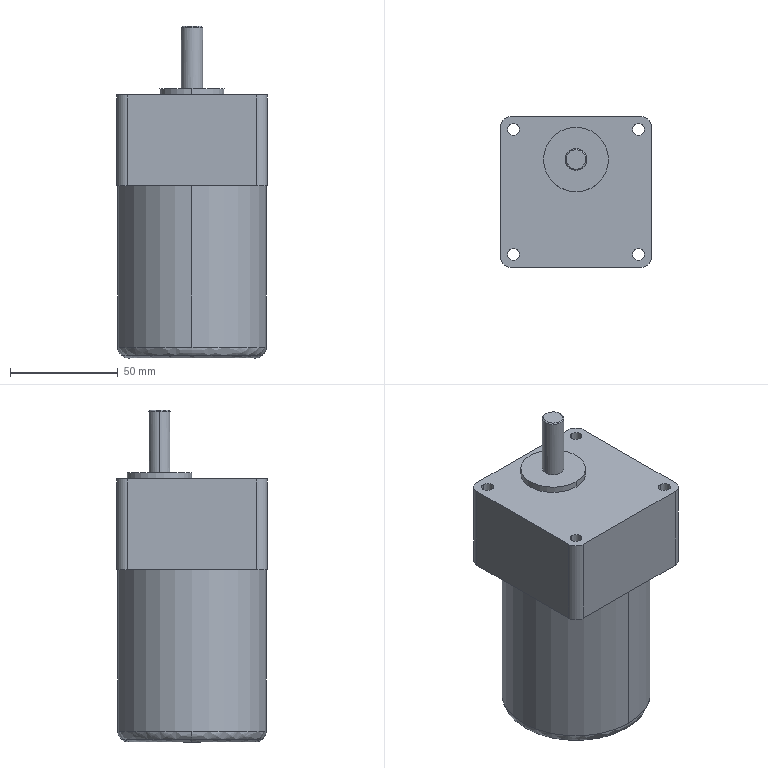Part | SolidWorks | features BaseBody 1 | 1 solid | 33 faces | box 70 x 70 x 154 mm | volume 503318 mm3 | cylinder 18 | plane 9 | spline 4 | cone 2 | commonest cylinder face diameters 5.5 x8 10 x6 30 x2 69 x2
STEP:
#1=CARTESIAN_POINT('',(180.25,352.,-74.5));
#2=VERTEX_POINT('',#1);
#3=CARTESIAN_POINT('',(239.25,352.,-74.5));
#4=VERTEX_POINT('',#3);
#5=CARTESIAN_POINT('',(180.25,352.,-74.5));
#6=CARTESIAN_POINT('',(180.25,353.933,-74.5));
#7=CARTESIAN_POINT('',(180.44,355.861,-74.5));
#8=CARTESIAN_POINT('',(181.194,359.65,-74.5));
#9=CARTESIAN_POINT('',(181.756,361.505,-74.5));
#10=CARTESIAN_POINT('',(183.235,365.074,-74.5));
#11=CARTESIAN_POINT('',(184.149,366.783,-74.5));
#12=CARTESIAN_POINT('',(186.295,369.995,-74.5));
#13=CARTESIAN_POINT('',(187.525,371.494,-74.5));
#14=CARTESIAN_POINT('',(190.256,374.226,-74.5));
#15=CARTESIAN_POINT('',(191.755,375.455,-74.5));
#16=CARTESIAN_POINT('',(194.967,377.602,-74.5));
#17=CARTESIAN_POINT('',(196.676,378.515,-74.5));
#18=CARTESIAN_POINT('',(200.245,379.994,-74.5));
#19=CARTESIAN_POINT('',(202.1,380.556,-74.5));
#20=CARTESIAN_POINT('',(205.889,381.31,-74.5));
#21=CARTESIAN_POINT('',(207.818,381.5,-74.5));
#22=CARTESIAN_POINT('',(211.682,381.5,-74.5));
#23=CARTESIAN_POINT('',(213.611,381.31,-74.5));
#24=CARTESIAN_POINT('',(217.4,380.556,-74.5));
#25=CARTESIAN_POINT('',(219.255,379.994,-74.5));
#26=CARTESIAN_POINT('',(222.824,378.515,-74.5));
#27=CARTESIAN_POINT('',(224.533,377.601,-74.5));
#28=CARTESIAN_POINT('',(227.745,375.455,-74.5));
#29=CARTESIAN_POINT('',(229.244,374.225,-74.5));
#30=CARTESIAN_POINT('',(231.976,371.494,-74.5));
#31=CARTESIAN_POINT('',(233.205,369.995,-74.5));
#32=CARTESIAN_POINT('',(235.352,366.783,-74.5));
#33=CARTESIAN_POINT('',(236.265,365.074,-74.5));
#34=CARTESIAN_POINT('',(237.744,361.505,-74.5));
#35=CARTESIAN_POINT('',(238.306,359.65,-74.5));
#36=CARTESIAN_POINT('',(239.06,355.861,-74.5));
#37=CARTESIAN_POINT('',(239.25,353.933,-74.5));
#38=CARTESIAN_POINT('',(239.25,352.,-74.5));
#39=B_SPLINE_CURVE_WITH_KNOTS('',3,(#5,#6,#7,#8,#9,#10,#11,#12,#13,#14,#15,#16,#17,#18,#19,#20,#21,#22,#23,#24,#25,#26,#27,#28,#29,#30,#31,#32,#33,#34,#35,#36,#37,#38),.UNSPECIFIED.,.F.,.F.,(4,2,2,2,2,2,2,2,2,2,2,2,2,2,2,2,4),(0.,0.0625,0.125,0.1875,0.25,0.3125,0.375,0.4375,0.5,0.5625,0.625,0.6875,0.75,0.8125,0.875,0.9375,1.),.UNSPECIFIED.);
#40=EDGE_CURVE('',#2,#4,#39,.T.);
#41=ORIENTED_EDGE('',*,*,#40,.F.);
#42=CARTESIAN_POINT('',(176.873,352.,-73.187));
#43=VERTEX_POINT('',#42);
#44=CARTESIAN_POINT('',(180.25,352.,-69.5));
#45=DIRECTION('',(0.,1.,0.));
#46=DIRECTION('',(-0.6754,0.,-0.7375));
#47=AXIS2_PLACEMENT_3D('',#44,#45,#46);
#48=CIRCLE('',#47,5.);
#49=EDGE_CURVE('',#2,#43,#48,.T.);
#50=ORIENTED_EDGE('',*,*,#49,.T.);
#51=CARTESIAN_POINT('',(242.627,352.,-73.187));
#52=VERTEX_POINT('',#51);
#53=CARTESIAN_POINT('',(209.75,352.,-73.187));
#54=DIRECTION('',(0.,0.,1.));
#55=DIRECTION('',(1.,0.,0.));
#56=AXIS2_PLACEMENT_3D('',#53,#54,#55);
#57=CIRCLE('',#56,32.877);
#58=EDGE_CURVE('',#52,#43,#57,.T.);
#59=ORIENTED_EDGE('',*,*,#58,.F.);
#60=CARTESIAN_POINT('',(239.25,352.,-69.5));
#61=DIRECTION('',(0.,-1.,0.));
#62=DIRECTION('',(0.6754,0.,-0.7375));
#63=AXIS2_PLACEMENT_3D('',#60,#61,#62);
#64=CIRCLE('',#63,5.);
#65=EDGE_CURVE('',#4,#52,#64,.T.);
#66=ORIENTED_EDGE('',*,*,#65,.F.);
#67=EDGE_LOOP('',(#41,#50,#59,#66));
#68=FACE_OUTER_BOUND('',#67,.T.);
#69=CARTESIAN_POINT('',(239.25,352.,-74.5));
#70=CARTESIAN_POINT('',(239.25,411.,-74.5));
#71=CARTESIAN_POINT('',(180.25,411.,-74.5));
#72=CARTESIAN_POINT('',(180.25,352.,-74.5));
#73=CARTESIAN_POINT('',(240.515,352.,-74.5));
#74=CARTESIAN_POINT('',(240.515,413.53,-74.5));
#75=CARTESIAN_POINT('',(178.985,413.53,-74.5));
#76=CARTESIAN_POINT('',(178.985,352.,-74.5));
#77=CARTESIAN_POINT('',(241.694,352.,-74.042));
#78=CARTESIAN_POINT('',(241.694,415.888,-74.042));
#79=CARTESIAN_POINT('',(177.806,415.888,-74.042));
#80=CARTESIAN_POINT('',(177.806,352.,-74.042));
#81=CARTESIAN_POINT('',(242.627,352.,-73.187));
#82=CARTESIAN_POINT('',(242.627,417.754,-73.187));
#83=CARTESIAN_POINT('',(176.873,417.754,-73.187));
#84=CARTESIAN_POINT('',(176.873,352.,-73.187));
#85=(BOUNDED_SURFACE()B_SPLINE_SURFACE(3,3,((#69,#70,#71,#72),(#73,#74,#75,#76),(#77,#78,#79,#80),(#81,#82,#83,#84)),.UNSPECIFIED.,.F.,.F.,.F.)B_SPLINE_SURFACE_WITH_KNOTS((4,4),(4,4),(0.,1.),(0.,1.),.UNSPECIFIED.)GEOMETRIC_REPRESENTATION_ITEM()RATIONAL_B_SPLINE_SURFACE(((1.,0.3333,0.3333,1.),(0.9547,0.3182,0.3182,0.9547),(0.9547,0.3182,0.3182,0.9547),(1.,0.3333,0.3333,1.)))REPRESENTATION_ITEM('')SURFACE());
#86=ADVANCED_FACE('',(#68),#85,.F.);
#87=ORIENTED_EDGE('',*,*,#58,.T.);
#88=CARTESIAN_POINT('',(175.25,352.,-69.5));
#89=VERTEX_POINT('',#88);
#90=CARTESIAN_POINT('',(180.25,352.,-69.5));
#91=DIRECTION('',(0.,1.,0.));
#92=DIRECTION('',(-0.6754,0.,-0.7375));
#93=AXIS2_PLACEMENT_3D('',#90,#91,#92);
#94=CIRCLE('',#93,5.);
#95=EDGE_CURVE('',#43,#89,#94,.T.);
#96=ORIENTED_EDGE('',*,*,#95,.T.);
#97=CARTESIAN_POINT('',(209.75,386.5,-69.5));
#98=VERTEX_POINT('',#97);
#99=CARTESIAN_POINT('',(209.75,352.,-69.5));
#100=DIRECTION('',(0.,0.,-1.));
#101=DIRECTION('',(1.,0.,0.));
#102=AXIS2_PLACEMENT_3D('',#99,#100,#101);
#103=CIRCLE('',#102,34.5);
#104=EDGE_CURVE('',#89,#98,#103,.T.);
#105=ORIENTED_EDGE('',*,*,#104,.T.);
#106=CARTESIAN_POINT('',(244.25,352.,-69.5));
#107=VERTEX_POINT('',#106);
#108=CARTESIAN_POINT('',(209.75,352.,-69.5));
#109=DIRECTION('',(0.,0.,-1.));
#110=DIRECTION('',(1.,0.,0.));
#111=AXIS2_PLACEMENT_3D('',#108,#109,#110);
#112=CIRCLE('',#111,34.5);
#113=EDGE_CURVE('',#98,#107,#112,.T.);
#114=ORIENTED_EDGE('',*,*,#113,.T.);
#115=CARTESIAN_POINT('',(239.25,352.,-69.5));
#116=DIRECTION('',(0.,-1.,0.));
#117=DIRECTION('',(0.6754,0.,-0.7375));
#118=AXIS2_PLACEMENT_3D('',#115,#116,#117);
#119=CIRCLE('',#118,5.);
#120=EDGE_CURVE('',#52,#107,#119,.T.);
#121=ORIENTED_EDGE('',*,*,#120,.F.);
#122=EDGE_LOOP('',(#87,#96,#105,#114,#121));
#123=FACE_OUTER_BOUND('',#122,.T.);
#124=CARTESIAN_POINT('',(242.627,352.,-73.187));
#125=CARTESIAN_POINT('',(242.627,417.754,-73.187));
#126=CARTESIAN_POINT('',(176.873,417.754,-73.187));
#127=CARTESIAN_POINT('',(176.873,352.,-73.187));
#128=CARTESIAN_POINT('',(243.677,352.,-72.226));
#129=CARTESIAN_POINT('',(243.677,419.853,-72.226));
#130=CARTESIAN_POINT('',(175.823,419.853,-72.226));
#131=CARTESIAN_POINT('',(175.823,352.,-72.226));
#132=CARTESIAN_POINT('',(244.25,352.,-70.923));
#133=CARTESIAN_POINT('',(244.25,421.,-70.923));
#134=CARTESIAN_POINT('',(175.25,421.,-70.923));
#135=CARTESIAN_POINT('',(175.25,352.,-70.923));
#136=CARTESIAN_POINT('',(244.25,352.,-69.5));
#137=CARTESIAN_POINT('',(244.25,421.,-69.5));
#138=CARTESIAN_POINT('',(175.25,421.,-69.5));
#139=CARTESIAN_POINT('',(175.25,352.,-69.5));
#140=(BOUNDED_SURFACE()B_SPLINE_SURFACE(3,3,((#124,#125,#126,#127),(#128,#129,#130,#131),(#132,#133,#134,#135),(#136,#137,#138,#139)),.UNSPECIFIED.,.F.,.F.,.F.)B_SPLINE_SURFACE_WITH_KNOTS((4,4),(4,4),(0.,1.),(0.,1.),.UNSPECIFIED.)GEOMETRIC_REPRESENTATION_ITEM()RATIONAL_B_SPLINE_SURFACE(((1.,0.3333,0.3333,1.),(0.9435,0.3145,0.3145,0.9435),(0.9435,0.3145,0.3145,0.9435),(1.,0.3333,0.3333,1.)))REPRESENTATION_ITEM('')SURFACE());
#141=ADVANCED_FACE('',(#123),#140,.F.);
#142=CARTESIAN_POINT('',(209.75,362.5,79.5));
#143=VERTEX_POINT('',#142);
#144=CARTESIAN_POINT('',(209.75,371.5,79.5));
#145=VERTEX_POINT('',#144);
#146=CARTESIAN_POINT('',(209.75,367.,79.5));
#147=DIRECTION('',(0.,0.,1.));
#148=DIRECTION('',(0.,1.,0.));
#149=AXIS2_PLACEMENT_3D('',#146,#147,#148);
#150=CIRCLE('',#149,4.5);
#151=EDGE_CURVE('',#143,#145,#150,.T.);
#152=ORIENTED_EDGE('',*,*,#151,.F.);
#153=CARTESIAN_POINT('',(209.75,362.,79.));
#154=VERTEX_POINT('',#153);
#155=CARTESIAN_POINT('',(209.75,362.5,79.5));
#156=DIRECTION('',(0.,-0.7071,-0.7071));
#157=VECTOR('',#156,1000.);
#158=LINE('',#155,#157);
#159=EDGE_CURVE('',#143,#154,#158,.T.);
#160=ORIENTED_EDGE('',*,*,#159,.T.);
#161=CARTESIAN_POINT('',(214.75,367.,79.));
#162=VERTEX_POINT('',#161);
#163=CARTESIAN_POINT('',(209.75,367.,79.));
#164=DIRECTION('',(0.,0.,-1.));
#165=DIRECTION('',(-1.,0.,0.));
#166=AXIS2_PLACEMENT_3D('',#163,#164,#165);
#167=CIRCLE('',#166,5.);
#168=EDGE_CURVE('',#162,#154,#167,.T.);
#169=ORIENTED_EDGE('',*,*,#168,.F.);
#170=CARTESIAN_POINT('',(209.75,372.,79.));
#171=VERTEX_POINT('',#170);
#172=CARTESIAN_POINT('',(209.75,367.,79.));
#173=DIRECTION('',(0.,0.,-1.));
#174=DIRECTION('',(-1.,0.,0.));
#175=AXIS2_PLACEMENT_3D('',#172,#173,#174);
#176=CIRCLE('',#175,5.);
#177=EDGE_CURVE('',#171,#162,#176,.T.);
#178=ORIENTED_EDGE('',*,*,#177,.F.);
#179=CARTESIAN_POINT('',(209.75,371.5,79.5));
#180=DIRECTION('',(0.,0.7071,-0.7071));
#181=VECTOR('',#180,1000.);
#182=LINE('',#179,#181);
#183=EDGE_CURVE('',#145,#171,#182,.T.);
#184=ORIENTED_EDGE('',*,*,#183,.F.);
#185=EDGE_LOOP('',(#152,#160,#169,#178,#184));
#186=FACE_OUTER_BOUND('',#185,.T.);
#187=CARTESIAN_POINT('',(209.75,367.,79.5));
#188=DIRECTION('',(0.,0.,-1.));
#189=DIRECTION('',(0.,1.,0.));
#190=AXIS2_PLACEMENT_3D('',#187,#188,#189);
#191=CONICAL_SURFACE('',#190,4.5,0.7854);
#192=ADVANCED_FACE('',(#186),#191,.T.);
#193=CARTESIAN_POINT('',(204.75,367.,50.5));
#194=VERTEX_POINT('',#193);
#195=CARTESIAN_POINT('',(214.75,367.,50.5));
#196=VERTEX_POINT('',#195);
#197=CARTESIAN_POINT('',(209.75,367.,50.5));
#198=DIRECTION('',(0.,0.,-1.));
#199=DIRECTION('',(1.,0.,0.));
#200=AXIS2_PLACEMENT_3D('',#197,#198,#199);
#201=CIRCLE('',#200,5.);
#202=EDGE_CURVE('',#194,#196,#201,.T.);
#203=ORIENTED_EDGE('',*,*,#202,.F.);
#204=CARTESIAN_POINT('',(204.75,367.,79.));
#205=VERTEX_POINT('',#204);
#206=CARTESIAN_POINT('',(204.75,367.,50.5));
#207=DIRECTION('',(0.,0.,1.));
#208=VECTOR('',#207,1000.);
#209=LINE('',#206,#208);
#210=EDGE_CURVE('',#194,#205,#209,.T.);
#211=ORIENTED_EDGE('',*,*,#210,.T.);
#212=CARTESIAN_POINT('',(209.75,367.,79.));
#213=DIRECTION('',(0.,0.,-1.));
#214=DIRECTION('',(-1.,0.,0.));
#215=AXIS2_PLACEMENT_3D('',#212,#213,#214);
#216=CIRCLE('',#215,5.);
#217=EDGE_CURVE('',#205,#171,#216,.T.);
#218=ORIENTED_EDGE('',*,*,#217,.T.);
#219=ORIENTED_EDGE('',*,*,#177,.T.);
#220=CARTESIAN_POINT('',(214.75,367.,50.5));
#221=DIRECTION('',(0.,0.,1.));
#222=VECTOR('',#221,1000.);
#223=LINE('',#220,#222);
#224=EDGE_CURVE('',#196,#162,#223,.T.);
#225=ORIENTED_EDGE('',*,*,#224,.F.);
#226=EDGE_LOOP('',(#203,#211,#218,#219,#225));
#227=FACE_OUTER_BOUND('',#226,.T.);
#228=CARTESIAN_POINT('',(209.75,367.,50.5));
#229=DIRECTION('',(0.,0.,1.));
#230=DIRECTION('',(1.,0.,0.));
#231=AXIS2_PLACEMENT_3D('',#228,#229,#230);
#232=CYLINDRICAL_SURFACE('',#231,5.);
#233=ADVANCED_FACE('',(#227),#232,.T.);
#234=CARTESIAN_POINT('',(209.75,382.,47.5));
#235=VERTEX_POINT('',#234);
#236=CARTESIAN_POINT('',(209.75,352.,47.5));
#237=VERTEX_POINT('',#236);
#238=CARTESIAN_POINT('',(209.75,367.,47.5));
#239=DIRECTION('',(0.,0.,-1.));
#240=DIRECTION('',(0.,-1.,0.));
#241=AXIS2_PLACEMENT_3D('',#238,#239,#240);
#242=CIRCLE('',#241,15.);
#243=EDGE_CURVE('',#235,#237,#242,.T.);
#244=ORIENTED_EDGE('',*,*,#243,.F.);
#245=CARTESIAN_POINT('',(209.75,382.,50.5));
#246=VERTEX_POINT('',#245);
#247=CARTESIAN_POINT('',(209.75,382.,47.5));
#248=DIRECTION('',(0.,0.,1.));
#249=VECTOR('',#248,1000.);
#250=LINE('',#247,#249);
#251=EDGE_CURVE('',#235,#246,#250,.T.);
#252=ORIENTED_EDGE('',*,*,#251,.T.);
#253=CARTESIAN_POINT('',(209.75,352.,50.5));
#254=VERTEX_POINT('',#253);
#255=CARTESIAN_POINT('',(209.75,367.,50.5));
#256=DIRECTION('',(0.,0.,-1.));
#257=DIRECTION('',(0.,-1.,0.));
#258=AXIS2_PLACEMENT_3D('',#255,#256,#257);
#259=CIRCLE('',#258,15.);
#260=EDGE_CURVE('',#246,#254,#259,.T.);
#261=ORIENTED_EDGE('',*,*,#260,.T.);
#262=CARTESIAN_POINT('',(209.75,352.,47.5));
#263=DIRECTION('',(0.,0.,1.));
#264=VECTOR('',#263,1000.);
#265=LINE('',#262,#264);
#266=EDGE_CURVE('',#237,#254,#265,.T.);
#267=ORIENTED_EDGE('',*,*,#266,.F.);
#268=EDGE_LOOP('',(#244,#252,#261,#267));
#269=FACE_OUTER_BOUND('',#268,.T.);
#270=CARTESIAN_POINT('',(209.75,367.,47.5));
#271=DIRECTION('',(0.,0.,1.));
#272=DIRECTION('',(0.,-1.,0.));
#273=AXIS2_PLACEMENT_3D('',#270,#271,#272);
#274=CYLINDRICAL_SURFACE('',#273,15.);
#275=ADVANCED_FACE('',(#269),#274,.T.);
#276=CARTESIAN_POINT('',(238.741,378.241,47.5));
#277=VERTEX_POINT('',#276);
#278=CARTESIAN_POINT('',(238.741,383.741,47.5));
#279=VERTEX_POINT('',#278);
#280=CARTESIAN_POINT('',(238.741,380.991,47.5));
#281=DIRECTION('',(0.,0.,-1.));
#282=DIRECTION('',(0.,1.,0.));
#283=AXIS2_PLACEMENT_3D('',#280,#281,#282);
#284=CIRCLE('',#283,2.75);
#285=EDGE_CURVE('',#277,#279,#284,.T.);
#286=ORIENTED_EDGE('',*,*,#285,.F.);
#287=CARTESIAN_POINT('',(238.741,378.241,5.5));
#288=VERTEX_POINT('',#287);
#289=CARTESIAN_POINT('',(238.741,378.241,47.5));
#290=DIRECTION('',(0.,0.,-1.));
#291=VECTOR('',#290,1000.);
#292=LINE('',#289,#291);
#293=EDGE_CURVE('',#277,#288,#292,.T.);
#294=ORIENTED_EDGE('',*,*,#293,.T.);
#295=CARTESIAN_POINT('',(238.741,383.741,5.5));
#296=VERTEX_POINT('',#295);
#297=CARTESIAN_POINT('',(238.741,380.991,5.5));
#298=DIRECTION('',(0.,0.,-1.));
#299=DIRECTION('',(0.,1.,0.));
#300=AXIS2_PLACEMENT_3D('',#297,#298,#299);
#301=CIRCLE('',#300,2.75);
#302=EDGE_CURVE('',#288,#296,#301,.T.);
#303=ORIENTED_EDGE('',*,*,#302,.T.);
#304=CARTESIAN_POINT('',(238.741,383.741,47.5));
#305=DIRECTION('',(0.,0.,-1.));
#306=VECTOR('',#305,1000.);
#307=LINE('',#304,#306);
#308=EDGE_CURVE('',#279,#296,#307,.T.);
#309=ORIENTED_EDGE('',*,*,#308,.F.);
#310=EDGE_LOOP('',(#286,#294,#303,#309));
#311=FACE_OUTER_BOUND('',#310,.T.);
#312=CARTESIAN_POINT('',(238.741,380.991,47.5));
#313=DIRECTION('',(0.,0.,-1.));
#314=DIRECTION('',(0.,1.,0.));
#315=AXIS2_PLACEMENT_3D('',#312,#313,#314);
#316=CYLINDRICAL_SURFACE('',#315,2.75);
#317=ADVANCED_FACE('',(#311),#316,.F.);
#318=CARTESIAN_POINT('',(238.741,320.259,47.5));
#319=VERTEX_POINT('',#318);
#320=CARTESIAN_POINT('',(238.741,325.759,47.5));
#321=VERTEX_POINT('',#320);
#322=CARTESIAN_POINT('',(238.741,323.009,47.5));
#323=DIRECTION('',(0.,0.,-1.));
#324=DIRECTION('',(0.,1.,0.));
#325=AXIS2_PLACEMENT_3D('',#322,#323,#324);
#326=CIRCLE('',#325,2.75);
#327=EDGE_CURVE('',#319,#321,#326,.T.);
#328=ORIENTED_EDGE('',*,*,#327,.F.);
#329=CARTESIAN_POINT('',(238.741,320.259,5.5));
#330=VERTEX_POINT('',#329);
#331=CARTESIAN_POINT('',(238.741,320.259,47.5));
#332=DIRECTION('',(0.,0.,-1.));
#333=VECTOR('',#332,1000.);
#334=LINE('',#331,#333);
#335=EDGE_CURVE('',#319,#330,#334,.T.);
#336=ORIENTED_EDGE('',*,*,#335,.T.);
#337=CARTESIAN_POINT('',(238.741,325.759,5.5));
#338=VERTEX_POINT('',#337);
#339=CARTESIAN_POINT('',(238.741,323.009,5.5));
#340=DIRECTION('',(0.,0.,-1.));
#341=DIRECTION('',(0.,1.,0.));
#342=AXIS2_PLACEMENT_3D('',#339,#340,#341);
#343=CIRCLE('',#342,2.75);
#344=EDGE_CURVE('',#330,#338,#343,.T.);
#345=ORIENTED_EDGE('',*,*,#344,.T.);
#346=CARTESIAN_POINT('',(238.741,325.759,47.5));
#347=DIRECTION('',(0.,0.,-1.));
#348=VECTOR('',#347,1000.);
#349=LINE('',#346,#348);
#350=EDGE_CURVE('',#321,#338,#349,.T.);
#351=ORIENTED_EDGE('',*,*,#350,.F.);
#352=EDGE_LOOP('',(#328,#336,#345,#351));
#353=FACE_OUTER_BOUND('',#352,.T.);
#354=CARTESIAN_POINT('',(238.741,323.009,47.5));
#355=DIRECTION('',(0.,0.,-1.));
#356=DIRECTION('',(0.,1.,0.));
#357=AXIS2_PLACEMENT_3D('',#354,#355,#356);
#358=CYLINDRICAL_SURFACE('',#357,2.75);
#359=ADVANCED_FACE('',(#353),#358,.F.);
#360=CARTESIAN_POINT('',(180.759,320.259,47.5));
#361=VERTEX_POINT('',#360);
#362=CARTESIAN_POINT('',(180.759,325.759,47.5));
#363=VERTEX_POINT('',#362);
#364=CARTESIAN_POINT('',(180.759,323.009,47.5));
#365=DIRECTION('',(0.,0.,-1.));
#366=DIRECTION('',(0.,1.,0.));
#367=AXIS2_PLACEMENT_3D('',#364,#365,#366);
#368=CIRCLE('',#367,2.75);
#369=EDGE_CURVE('',#361,#363,#368,.T.);
#370=ORIENTED_EDGE('',*,*,#369,.F.);
#371=CARTESIAN_POINT('',(180.759,320.259,5.5));
#372=VERTEX_POINT('',#371);
#373=CARTESIAN_POINT('',(180.759,320.259,47.5));
#374=DIRECTION('',(0.,0.,-1.));
#375=VECTOR('',#374,1000.);
#376=LINE('',#373,#375);
#377=EDGE_CURVE('',#361,#372,#376,.T.);
#378=ORIENTED_EDGE('',*,*,#377,.T.);
#379=CARTESIAN_POINT('',(180.759,325.759,5.5));
#380=VERTEX_POINT('',#379);
#381=CARTESIAN_POINT('',(180.759,323.009,5.5));
#382=DIRECTION('',(0.,0.,-1.));
#383=DIRECTION('',(0.,1.,0.));
#384=AXIS2_PLACEMENT_3D('',#381,#382,#383);
#385=CIRCLE('',#384,2.75);
#386=EDGE_CURVE('',#372,#380,#385,.T.);
#387=ORIENTED_EDGE('',*,*,#386,.T.);
#388=CARTESIAN_POINT('',(180.759,325.759,47.5));
#389=DIRECTION('',(0.,0.,-1.));
#390=VECTOR('',#389,1000.);
#391=LINE('',#388,#390);
#392=EDGE_CURVE('',#363,#380,#391,.T.);
#393=ORIENTED_EDGE('',*,*,#392,.F.);
#394=EDGE_LOOP('',(#370,#378,#387,#393));
#395=FACE_OUTER_BOUND('',#394,.T.);
#396=CARTESIAN_POINT('',(180.759,323.009,47.5));
#397=DIRECTION('',(0.,0.,-1.));
#398=DIRECTION('',(0.,1.,0.));
#399=AXIS2_PLACEMENT_3D('',#396,#397,#398);
#400=CYLINDRICAL_SURFACE('',#399,2.75);
#401=ADVANCED_FACE('',(#395),#400,.F.);
#402=CARTESIAN_POINT('',(180.759,378.241,47.5));
#403=VERTEX_POINT('',#402);
#404=CARTESIAN_POINT('',(180.759,383.741,47.5));
#405=VERTEX_POINT('',#404);
#406=CARTESIAN_POINT('',(180.759,380.991,47.5));
#407=DIRECTION('',(0.,0.,-1.));
#408=DIRECTION('',(0.,1.,0.));
#409=AXIS2_PLACEMENT_3D('',#406,#407,#408);
#410=CIRCLE('',#409,2.75);
#411=EDGE_CURVE('',#403,#405,#410,.T.);
#412=ORIENTED_EDGE('',*,*,#411,.F.);
#413=CARTESIAN_POINT('',(180.759,378.241,5.5));
#414=VERTEX_POINT('',#413);
#415=CARTESIAN_POINT('',(180.759,378.241,47.5));
#416=DIRECTION('',(0.,0.,-1.));
#417=VECTOR('',#416,1000.);
#418=LINE('',#415,#417);
#419=EDGE_CURVE('',#403,#414,#418,.T.);
#420=ORIENTED_EDGE('',*,*,#419,.T.);
#421=CARTESIAN_POINT('',(180.759,383.741,5.5));
#422=VERTEX_POINT('',#421);
#423=CARTESIAN_POINT('',(180.759,380.991,5.5));
#424=DIRECTION('',(0.,0.,-1.));
#425=DIRECTION('',(0.,1.,0.));
#426=AXIS2_PLACEMENT_3D('',#423,#424,#425);
#427=CIRCLE('',#426,2.75);
#428=EDGE_CURVE('',#414,#422,#427,.T.);
#429=ORIENTED_EDGE('',*,*,#428,.T.);
#430=CARTESIAN_POINT('',(180.759,383.741,47.5));
#431=DIRECTION('',(0.,0.,-1.));
#432=VECTOR('',#431,1000.);
#433=LINE('',#430,#432);
#434=EDGE_CURVE('',#405,#422,#433,.T.);
#435=ORIENTED_EDGE('',*,*,#434,.F.);
#436=EDGE_LOOP('',(#412,#420,#429,#435));
#437=FACE_OUTER_BOUND('',#436,.T.);
#438=CARTESIAN_POINT('',(180.759,380.991,47.5));
#439=DIRECTION('',(0.,0.,-1.));
#440=DIRECTION('',(0.,1.,0.));
#441=AXIS2_PLACEMENT_3D('',#438,#439,#440);
#442=CYLINDRICAL_SURFACE('',#441,2.75);
#443=ADVANCED_FACE('',(#437),#442,.F.);
#444=CARTESIAN_POINT('',(209.75,386.5,5.5));
#445=VERTEX_POINT('',#444);
#446=CARTESIAN_POINT('',(209.75,317.5,5.5));
#447=VERTEX_POINT('',#446);
#448=CARTESIAN_POINT('',(209.75,352.,5.5));
#449=DIRECTION('',(0.,0.,-1.));
#450=DIRECTION('',(0.,1.,0.));
#451=AXIS2_PLACEMENT_3D('',#448,#449,#450);
#452=CIRCLE('',#451,34.5);
#453=EDGE_CURVE('',#445,#447,#452,.T.);
#454=ORIENTED_EDGE('',*,*,#453,.T.);
#455=CARTESIAN_POINT('',(209.75,317.5,-69.5));
#456=VERTEX_POINT('',#455);
#457=CARTESIAN_POINT('',(209.75,317.5,5.5));
#458=DIRECTION('',(0.,0.,-1.));
#459=VECTOR('',#458,1000.);
#460=LINE('',#457,#459);
#461=EDGE_CURVE('',#447,#456,#460,.T.);
#462=ORIENTED_EDGE('',*,*,#461,.T.);
#463=CARTESIAN_POINT('',(209.75,352.,-69.5));
#464=DIRECTION('',(0.,0.,-1.));
#465=DIRECTION('',(1.,0.,0.));
#466=AXIS2_PLACEMENT_3D('',#463,#464,#465);
#467=CIRCLE('',#466,34.5);
#468=EDGE_CURVE('',#107,#456,#467,.T.);
#469=ORIENTED_EDGE('',*,*,#468,.F.);
#470=ORIENTED_EDGE('',*,*,#113,.F.);
#471=CARTESIAN_POINT('',(209.75,386.5,5.5));
#472=DIRECTION('',(0.,0.,-1.));
#473=VECTOR('',#472,1000.);
#474=LINE('',#471,#473);
#475=EDGE_CURVE('',#445,#98,#474,.T.);
#476=ORIENTED_EDGE('',*,*,#475,.F.);
#477=EDGE_LOOP('',(#454,#462,#469,#470,#476));
#478=FACE_OUTER_BOUND('',#477,.T.);
#479=CARTESIAN_POINT('',(209.75,352.,5.5));
#480=DIRECTION('',(0.,0.,-1.));
#481=DIRECTION('',(0.,1.,0.));
#482=AXIS2_PLACEMENT_3D('',#479,#480,#481);
#483=CYLINDRICAL_SURFACE('',#482,34.5);
#484=ADVANCED_FACE('',(#478),#483,.T.);
#485=ORIENTED_EDGE('',*,*,#95,.F.);
#486=CARTESIAN_POINT('',(209.75,352.,-73.187));
#487=DIRECTION('',(0.,0.,1.));
#488=DIRECTION('',(1.,0.,0.));
#489=AXIS2_PLACEMENT_3D('',#486,#487,#488);
#490=CIRCLE('',#489,32.877);
#491=EDGE_CURVE('',#43,#52,#490,.T.);
#492=ORIENTED_EDGE('',*,*,#491,.T.);
#493=ORIENTED_EDGE('',*,*,#120,.T.);
#494=ORIENTED_EDGE('',*,*,#468,.T.);
#495=CARTESIAN_POINT('',(209.75,352.,-69.5));
#496=DIRECTION('',(0.,0.,-1.));
#497=DIRECTION('',(1.,0.,0.));
#498=AXIS2_PLACEMENT_3D('',#495,#496,#497);
#499=CIRCLE('',#498,34.5);
#500=EDGE_CURVE('',#456,#89,#499,.T.);
#501=ORIENTED_EDGE('',*,*,#500,.T.);
#502=EDGE_LOOP('',(#485,#492,#493,#494,#501));
#503=FACE_OUTER_BOUND('',#502,.T.);
#504=CARTESIAN_POINT('',(176.873,352.,-73.187));
#505=CARTESIAN_POINT('',(176.873,286.246,-73.187));
#506=CARTESIAN_POINT('',(242.627,286.246,-73.187));
#507=CARTESIAN_POINT('',(242.627,352.,-73.187));
#508=CARTESIAN_POINT('',(175.823,352.,-72.226));
#509=CARTESIAN_POINT('',(175.823,284.147,-72.226));
#510=CARTESIAN_POINT('',(243.677,284.147,-72.226));
#511=CARTESIAN_POINT('',(243.677,352.,-72.226));
#512=CARTESIAN_POINT('',(175.25,352.,-70.923));
#513=CARTESIAN_POINT('',(175.25,283.,-70.923));
#514=CARTESIAN_POINT('',(244.25,283.,-70.923));
#515=CARTESIAN_POINT('',(244.25,352.,-70.923));
#516=CARTESIAN_POINT('',(175.25,352.,-69.5));
#517=CARTESIAN_POINT('',(175.25,283.,-69.5));
#518=CARTESIAN_POINT('',(244.25,283.,-69.5));
#519=CARTESIAN_POINT('',(244.25,352.,-69.5));
#520=(BOUNDED_SURFACE()B_SPLINE_SURFACE(3,3,((#504,#505,#506,#507),(#508,#509,#510,#511),(#512,#513,#514,#515),(#516,#517,#518,#519)),.UNSPECIFIED.,.F.,.F.,.F.)B_SPLINE_SURFACE_WITH_KNOTS((4,4),(4,4),(0.,1.),(0.,1.),.UNSPECIFIED.)GEOMETRIC_REPRESENTATION_ITEM()RATIONAL_B_SPLINE_SURFACE(((1.,0.3333,0.3333,1.),(0.9435,0.3145,0.3145,0.9435),(0.9435,0.3145,0.3145,0.9435),(1.,0.3333,0.3333,1.)))REPRESENTATION_ITEM('')SURFACE());
#521=ADVANCED_FACE('',(#503),#520,.F.);
#522=ORIENTED_EDGE('',*,*,#159,.F.);
#523=CARTESIAN_POINT('',(209.75,367.,79.5));
#524=DIRECTION('',(0.,0.,1.));
#525=DIRECTION('',(0.,1.,0.));
#526=AXIS2_PLACEMENT_3D('',#523,#524,#525);
#527=CIRCLE('',#526,4.5);
#528=EDGE_CURVE('',#145,#143,#527,.T.);
#529=ORIENTED_EDGE('',*,*,#528,.F.);
#530=ORIENTED_EDGE('',*,*,#183,.T.);
#531=ORIENTED_EDGE('',*,*,#217,.F.);
#532=CARTESIAN_POINT('',(209.75,367.,79.));
#533=DIRECTION('',(0.,0.,-1.));
#534=DIRECTION('',(-1.,0.,0.));
#535=AXIS2_PLACEMENT_3D('',#532,#533,#534);
#536=CIRCLE('',#535,5.);
#537=EDGE_CURVE('',#154,#205,#536,.T.);
#538=ORIENTED_EDGE('',*,*,#537,.F.);
#539=EDGE_LOOP('',(#522,#529,#530,#531,#538));
#540=FACE_OUTER_BOUND('',#539,.T.);
#541=CARTESIAN_POINT('',(209.75,367.,79.5));
#542=DIRECTION('',(0.,0.,-1.));
#543=DIRECTION('',(0.,1.,0.));
#544=AXIS2_PLACEMENT_3D('',#541,#542,#543);
#545=CONICAL_SURFACE('',#544,4.5,0.7854);
#546=ADVANCED_FACE('',(#540),#545,.T.);
#547=ORIENTED_EDGE('',*,*,#210,.F.);
#548=CARTESIAN_POINT('',(209.75,367.,50.5));
#549=DIRECTION('',(0.,0.,-1.));
#550=DIRECTION('',(1.,0.,0.));
#551=AXIS2_PLACEMENT_3D('',#548,#549,#550);
#552=CIRCLE('',#551,5.);
#553=EDGE_CURVE('',#196,#194,#552,.T.);
#554=ORIENTED_EDGE('',*,*,#553,.F.);
#555=ORIENTED_EDGE('',*,*,#224,.T.);
#556=ORIENTED_EDGE('',*,*,#168,.T.);
#557=ORIENTED_EDGE('',*,*,#537,.T.);
#558=EDGE_LOOP('',(#547,#554,#555,#556,#557));
#559=FACE_OUTER_BOUND('',#558,.T.);
#560=CARTESIAN_POINT('',(209.75,367.,50.5));
#561=DIRECTION('',(0.,0.,1.));
#562=DIRECTION('',(1.,0.,0.));
#563=AXIS2_PLACEMENT_3D('',#560,#561,#562);
#564=CYLINDRICAL_SURFACE('',#563,5.);
#565=ADVANCED_FACE('',(#559),#564,.T.);
#566=ORIENTED_EDGE('',*,*,#528,.T.);
#567=ORIENTED_EDGE('',*,*,#151,.T.);
#568=EDGE_LOOP('',(#566,#567));
#569=FACE_OUTER_BOUND('',#568,.T.);
#570=CARTESIAN_POINT('',(214.47,362.28,79.5));
#571=DIRECTION('',(0.,0.,-1.));
#572=DIRECTION('',(-1.,0.,0.));
#573=AXIS2_PLACEMENT_3D('',#570,#571,#572);
#574=PLANE('',#573);
#575=ADVANCED_FACE('',(#569),#574,.F.);
#576=ORIENTED_EDGE('',*,*,#553,.T.);
#577=ORIENTED_EDGE('',*,*,#202,.T.);
#578=EDGE_LOOP('',(#576,#577));
#579=FACE_BOUND('',#578,.T.);
#580=CARTESIAN_POINT('',(209.75,367.,50.5));
#581=DIRECTION('',(0.,0.,-1.));
#582=DIRECTION('',(0.,-1.,0.));
#583=AXIS2_PLACEMENT_3D('',#580,#581,#582);
#584=CIRCLE('',#583,15.);
#585=EDGE_CURVE('',#254,#246,#584,.T.);
#586=ORIENTED_EDGE('',*,*,#585,.F.);
#587=ORIENTED_EDGE('',*,*,#260,.F.);
#588=EDGE_LOOP('',(#586,#587));
#589=FACE_OUTER_BOUND('',#588,.T.);
#590=CARTESIAN_POINT('',(225.35,351.4,50.5));
#591=DIRECTION('',(0.,0.,-1.));
#592=DIRECTION('',(-1.,0.,0.));
#593=AXIS2_PLACEMENT_3D('',#590,#591,#592);
#594=PLANE('',#593);
#595=ADVANCED_FACE('',(#579,#589),#594,.F.);
#596=ORIENTED_EDGE('',*,*,#251,.F.);
#597=CARTESIAN_POINT('',(209.75,367.,47.5));
#598=DIRECTION('',(0.,0.,-1.));
#599=DIRECTION('',(0.,-1.,0.));
#600=AXIS2_PLACEMENT_3D('',#597,#598,#599);
#601=CIRCLE('',#600,15.);
#602=EDGE_CURVE('',#237,#235,#601,.T.);
#603=ORIENTED_EDGE('',*,*,#602,.F.);
#604=ORIENTED_EDGE('',*,*,#266,.T.);
#605=ORIENTED_EDGE('',*,*,#585,.T.);
#606=EDGE_LOOP('',(#596,#603,#604,#605));
#607=FACE_OUTER_BOUND('',#606,.T.);
#608=CARTESIAN_POINT('',(209.75,367.,47.5));
#609=DIRECTION('',(0.,0.,1.));
#610=DIRECTION('',(0.,-1.,0.));
#611=AXIS2_PLACEMENT_3D('',#608,#609,#610);
#612=CYLINDRICAL_SURFACE('',#611,15.);
#613=ADVANCED_FACE('',(#607),#612,.T.);
#614=ORIENTED_EDGE('',*,*,#602,.T.);
#615=ORIENTED_EDGE('',*,*,#243,.T.);
#616=EDGE_LOOP('',(#614,#615));
#617=FACE_BOUND('',#616,.T.);
#618=CARTESIAN_POINT('',(238.741,380.991,47.5));
#619=DIRECTION('',(0.,0.,-1.));
#620=DIRECTION('',(0.,1.,0.));
#621=AXIS2_PLACEMENT_3D('',#618,#619,#620);
#622=CIRCLE('',#621,2.75);
#623=EDGE_CURVE('',#279,#277,#622,.T.);
#624=ORIENTED_EDGE('',*,*,#623,.T.);
#625=ORIENTED_EDGE('',*,*,#285,.T.);
#626=EDGE_LOOP('',(#624,#625));
#627=FACE_BOUND('',#626,.T.);
#628=CARTESIAN_POINT('',(238.741,323.009,47.5));
#629=DIRECTION('',(0.,0.,-1.));
#630=DIRECTION('',(0.,1.,0.));
#631=AXIS2_PLACEMENT_3D('',#628,#629,#630);
#632=CIRCLE('',#631,2.75);
#633=EDGE_CURVE('',#321,#319,#632,.T.);
#634=ORIENTED_EDGE('',*,*,#633,.T.);
#635=ORIENTED_EDGE('',*,*,#327,.T.);
#636=EDGE_LOOP('',(#634,#635));
#637=FACE_BOUND('',#636,.T.);
#638=CARTESIAN_POINT('',(180.759,323.009,47.5));
#639=DIRECTION('',(0.,0.,-1.));
#640=DIRECTION('',(0.,1.,0.));
#641=AXIS2_PLACEMENT_3D('',#638,#639,#640);
#642=CIRCLE('',#641,2.75);
#643=EDGE_CURVE('',#363,#361,#642,.T.);
#644=ORIENTED_EDGE('',*,*,#643,.T.);
#645=ORIENTED_EDGE('',*,*,#369,.T.);
#646=EDGE_LOOP('',(#644,#645));
#647=FACE_BOUND('',#646,.T.);
#648=CARTESIAN_POINT('',(180.759,380.991,47.5));
#649=DIRECTION('',(0.,0.,-1.));
#650=DIRECTION('',(0.,1.,0.));
#651=AXIS2_PLACEMENT_3D('',#648,#649,#650);
#652=CIRCLE('',#651,2.75);
#653=EDGE_CURVE('',#405,#403,#652,.T.);
#654=ORIENTED_EDGE('',*,*,#653,.T.);
#655=ORIENTED_EDGE('',*,*,#411,.T.);
#656=EDGE_LOOP('',(#654,#655));
#657=FACE_BOUND('',#656,.T.);
#658=CARTESIAN_POINT('',(239.75,317.,47.5));
#659=VERTEX_POINT('',#658);
#660=CARTESIAN_POINT('',(244.75,322.,47.5));
#661=VERTEX_POINT('',#660);
#662=CARTESIAN_POINT('',(239.75,322.,47.5));
#663=DIRECTION('',(0.,0.,1.));
#664=DIRECTION('',(-1.,0.,0.));
#665=AXIS2_PLACEMENT_3D('',#662,#663,#664);
#666=CIRCLE('',#665,5.);
#667=EDGE_CURVE('',#659,#661,#666,.T.);
#668=ORIENTED_EDGE('',*,*,#667,.T.);
#669=CARTESIAN_POINT('',(244.75,382.,47.5));
#670=VERTEX_POINT('',#669);
#671=CARTESIAN_POINT('',(244.75,352.,47.5));
#672=DIRECTION('',(0.,1.,0.));
#673=VECTOR('',#672,1000.);
#674=LINE('',#671,#673);
#675=EDGE_CURVE('',#661,#670,#674,.T.);
#676=ORIENTED_EDGE('',*,*,#675,.T.);
#677=CARTESIAN_POINT('',(239.75,387.,47.5));
#678=VERTEX_POINT('',#677);
#679=CARTESIAN_POINT('',(239.75,382.,47.5));
#680=DIRECTION('',(0.,0.,1.));
#681=DIRECTION('',(-1.,0.,0.));
#682=AXIS2_PLACEMENT_3D('',#679,#680,#681);
#683=CIRCLE('',#682,5.);
#684=EDGE_CURVE('',#670,#678,#683,.T.);
#685=ORIENTED_EDGE('',*,*,#684,.T.);
#686=CARTESIAN_POINT('',(179.75,387.,47.5));
#687=VERTEX_POINT('',#686);
#688=CARTESIAN_POINT('',(209.75,387.,47.5));
#689=DIRECTION('',(-1.,0.,0.));
#690=VECTOR('',#689,1000.);
#691=LINE('',#688,#690);
#692=EDGE_CURVE('',#678,#687,#691,.T.);
#693=ORIENTED_EDGE('',*,*,#692,.T.);
#694=CARTESIAN_POINT('',(174.75,382.,47.5));
#695=VERTEX_POINT('',#694);
#696=CARTESIAN_POINT('',(179.75,382.,47.5));
#697=DIRECTION('',(0.,0.,1.));
#698=DIRECTION('',(1.,0.,0.));
#699=AXIS2_PLACEMENT_3D('',#696,#697,#698);
#700=CIRCLE('',#699,5.);
#701=EDGE_CURVE('',#687,#695,#700,.T.);
#702=ORIENTED_EDGE('',*,*,#701,.T.);
#703=CARTESIAN_POINT('',(174.75,322.,47.5));
#704=VERTEX_POINT('',#703);
#705=CARTESIAN_POINT('',(174.75,352.,47.5));
#706=DIRECTION('',(0.,-1.,0.));
#707=VECTOR('',#706,1000.);
#708=LINE('',#705,#707);
#709=EDGE_CURVE('',#695,#704,#708,.T.);
#710=ORIENTED_EDGE('',*,*,#709,.T.);
#711=CARTESIAN_POINT('',(179.75,317.,47.5));
#712=VERTEX_POINT('',#711);
#713=CARTESIAN_POINT('',(179.75,322.,47.5));
#714=DIRECTION('',(0.,0.,1.));
#715=DIRECTION('',(0.,1.,0.));
#716=AXIS2_PLACEMENT_3D('',#713,#714,#715);
#717=CIRCLE('',#716,5.);
#718=EDGE_CURVE('',#704,#712,#717,.T.);
#719=ORIENTED_EDGE('',*,*,#718,.T.);
#720=CARTESIAN_POINT('',(209.75,317.,47.5));
#721=DIRECTION('',(1.,0.,0.));
#722=VECTOR('',#721,1000.);
#723=LINE('',#720,#722);
#724=EDGE_CURVE('',#712,#659,#723,.T.);
#725=ORIENTED_EDGE('',*,*,#724,.T.);
#726=EDGE_LOOP('',(#668,#676,#685,#693,#702,#710,#719,#725));
#727=FACE_OUTER_BOUND('',#726,.T.);
#728=CARTESIAN_POINT('',(173.35,315.6,47.5));
#729=DIRECTION('',(0.,0.,1.));
#730=DIRECTION('',(1.,0.,0.));
#731=AXIS2_PLACEMENT_3D('',#728,#729,#730);
#732=PLANE('',#731);
#733=ADVANCED_FACE('',(#617,#627,#637,#647,#657,#727),#732,.T.);
#734=ORIENTED_EDGE('',*,*,#293,.F.);
#735=ORIENTED_EDGE('',*,*,#623,.F.);
#736=ORIENTED_EDGE('',*,*,#308,.T.);
#737=CARTESIAN_POINT('',(238.741,380.991,5.5));
#738=DIRECTION('',(0.,0.,-1.));
#739=DIRECTION('',(0.,1.,0.));
#740=AXIS2_PLACEMENT_3D('',#737,#738,#739);
#741=CIRCLE('',#740,2.75);
#742=EDGE_CURVE('',#296,#288,#741,.T.);
#743=ORIENTED_EDGE('',*,*,#742,.T.);
#744=EDGE_LOOP('',(#734,#735,#736,#743));
#745=FACE_OUTER_BOUND('',#744,.T.);
#746=CARTESIAN_POINT('',(238.741,380.991,47.5));
#747=DIRECTION('',(0.,0.,-1.));
#748=DIRECTION('',(0.,1.,0.));
#749=AXIS2_PLACEMENT_3D('',#746,#747,#748);
#750=CYLINDRICAL_SURFACE('',#749,2.75);
#751=ADVANCED_FACE('',(#745),#750,.F.);
#752=ORIENTED_EDGE('',*,*,#335,.F.);
#753=ORIENTED_EDGE('',*,*,#633,.F.);
#754=ORIENTED_EDGE('',*,*,#350,.T.);
#755=CARTESIAN_POINT('',(238.741,323.009,5.5));
#756=DIRECTION('',(0.,0.,-1.));
#757=DIRECTION('',(0.,1.,0.));
#758=AXIS2_PLACEMENT_3D('',#755,#756,#757);
#759=CIRCLE('',#758,2.75);
#760=EDGE_CURVE('',#338,#330,#759,.T.);
#761=ORIENTED_EDGE('',*,*,#760,.T.);
#762=EDGE_LOOP('',(#752,#753,#754,#761));
#763=FACE_OUTER_BOUND('',#762,.T.);
#764=CARTESIAN_POINT('',(238.741,323.009,47.5));
#765=DIRECTION('',(0.,0.,-1.));
#766=DIRECTION('',(0.,1.,0.));
#767=AXIS2_PLACEMENT_3D('',#764,#765,#766);
#768=CYLINDRICAL_SURFACE('',#767,2.75);
#769=ADVANCED_FACE('',(#763),#768,.F.);
#770=ORIENTED_EDGE('',*,*,#377,.F.);
#771=ORIENTED_EDGE('',*,*,#643,.F.);
#772=ORIENTED_EDGE('',*,*,#392,.T.);
#773=CARTESIAN_POINT('',(180.759,323.009,5.5));
#774=DIRECTION('',(0.,0.,-1.));
#775=DIRECTION('',(0.,1.,0.));
#776=AXIS2_PLACEMENT_3D('',#773,#774,#775);
#777=CIRCLE('',#776,2.75);
#778=EDGE_CURVE('',#380,#372,#777,.T.);
#779=ORIENTED_EDGE('',*,*,#778,.T.);
#780=EDGE_LOOP('',(#770,#771,#772,#779));
#781=FACE_OUTER_BOUND('',#780,.T.);
#782=CARTESIAN_POINT('',(180.759,323.009,47.5));
#783=DIRECTION('',(0.,0.,-1.));
#784=DIRECTION('',(0.,1.,0.));
#785=AXIS2_PLACEMENT_3D('',#782,#783,#784);
#786=CYLINDRICAL_SURFACE('',#785,2.75);
#787=ADVANCED_FACE('',(#781),#786,.F.);
#788=ORIENTED_EDGE('',*,*,#419,.F.);
#789=ORIENTED_EDGE('',*,*,#653,.F.);
#790=ORIENTED_EDGE('',*,*,#434,.T.);
#791=CARTESIAN_POINT('',(180.759,380.991,5.5));
#792=DIRECTION('',(0.,0.,-1.));
#793=DIRECTION('',(0.,1.,0.));
#794=AXIS2_PLACEMENT_3D('',#791,#792,#793);
#795=CIRCLE('',#794,2.75);
#796=EDGE_CURVE('',#422,#414,#795,.T.);
#797=ORIENTED_EDGE('',*,*,#796,.T.);
#798=EDGE_LOOP('',(#788,#789,#790,#797));
#799=FACE_OUTER_BOUND('',#798,.T.);
#800=CARTESIAN_POINT('',(180.759,380.991,47.5));
#801=DIRECTION('',(0.,0.,-1.));
#802=DIRECTION('',(0.,1.,0.));
#803=AXIS2_PLACEMENT_3D('',#800,#801,#802);
#804=CYLINDRICAL_SURFACE('',#803,2.75);
#805=ADVANCED_FACE('',(#799),#804,.F.);
#806=CARTESIAN_POINT('',(244.75,322.,5.5));
#807=VERTEX_POINT('',#806);
#808=CARTESIAN_POINT('',(244.75,322.,26.5));
#809=DIRECTION('',(0.,0.,-1.));
#810=VECTOR('',#809,1000.);
#811=LINE('',#808,#810);
#812=EDGE_CURVE('',#661,#807,#811,.T.);
#813=ORIENTED_EDGE('',*,*,#812,.T.);
#814=CARTESIAN_POINT('',(244.75,382.,5.5));
#815=VERTEX_POINT('',#814);
#816=CARTESIAN_POINT('',(244.75,352.,5.5));
#817=DIRECTION('',(0.,1.,0.));
#818=VECTOR('',#817,1000.);
#819=LINE('',#816,#818);
#820=EDGE_CURVE('',#807,#815,#819,.T.);
#821=ORIENTED_EDGE('',*,*,#820,.T.);
#822=CARTESIAN_POINT('',(244.75,382.,26.5));
#823=DIRECTION('',(0.,0.,1.));
#824=VECTOR('',#823,1000.);
#825=LINE('',#822,#824);
#826=EDGE_CURVE('',#815,#670,#825,.T.);
#827=ORIENTED_EDGE('',*,*,#826,.T.);
#828=ORIENTED_EDGE('',*,*,#675,.F.);
#829=EDGE_LOOP('',(#813,#821,#827,#828));
#830=FACE_OUTER_BOUND('',#829,.T.);
#831=CARTESIAN_POINT('',(244.75,320.8,48.34));
#832=DIRECTION('',(1.,0.,0.));
#833=DIRECTION('',(0.,0.,-1.));
#834=AXIS2_PLACEMENT_3D('',#831,#832,#833);
#835=PLANE('',#834);
#836=ADVANCED_FACE('',(#830),#835,.T.);
#837=ORIENTED_EDGE('',*,*,#667,.F.);
#838=CARTESIAN_POINT('',(239.75,317.,5.5));
#839=VERTEX_POINT('',#838);
#840=CARTESIAN_POINT('',(239.75,317.,26.5));
#841=DIRECTION('',(0.,0.,1.));
#842=VECTOR('',#841,1000.);
#843=LINE('',#840,#842);
#844=EDGE_CURVE('',#839,#659,#843,.T.);
#845=ORIENTED_EDGE('',*,*,#844,.F.);
#846=CARTESIAN_POINT('',(239.75,322.,5.5));
#847=DIRECTION('',(0.,0.,-1.));
#848=DIRECTION('',(-1.,0.,0.));
#849=AXIS2_PLACEMENT_3D('',#846,#847,#848);
#850=CIRCLE('',#849,5.);
#851=EDGE_CURVE('',#807,#839,#850,.T.);
#852=ORIENTED_EDGE('',*,*,#851,.F.);
#853=ORIENTED_EDGE('',*,*,#812,.F.);
#854=EDGE_LOOP('',(#837,#845,#852,#853));
#855=FACE_OUTER_BOUND('',#854,.T.);
#856=CARTESIAN_POINT('',(239.75,322.,47.5));
#857=DIRECTION('',(0.,0.,-1.));
#858=DIRECTION('',(-1.,0.,0.));
#859=AXIS2_PLACEMENT_3D('',#856,#857,#858);
#860=CYLINDRICAL_SURFACE('',#859,5.);
#861=ADVANCED_FACE('',(#855),#860,.T.);
#862=CARTESIAN_POINT('',(179.75,317.,5.5));
#863=VERTEX_POINT('',#862);
#864=CARTESIAN_POINT('',(179.75,317.,26.5));
#865=DIRECTION('',(0.,0.,-1.));
#866=VECTOR('',#865,1000.);
#867=LINE('',#864,#866);
#868=EDGE_CURVE('',#712,#863,#867,.T.);
#869=ORIENTED_EDGE('',*,*,#868,.T.);
#870=CARTESIAN_POINT('',(209.75,317.,5.5));
#871=DIRECTION('',(1.,0.,0.));
#872=VECTOR('',#871,1000.);
#873=LINE('',#870,#872);
#874=EDGE_CURVE('',#863,#839,#873,.T.);
#875=ORIENTED_EDGE('',*,*,#874,.T.);
#876=ORIENTED_EDGE('',*,*,#844,.T.);
#877=ORIENTED_EDGE('',*,*,#724,.F.);
#878=EDGE_LOOP('',(#869,#875,#876,#877));
#879=FACE_OUTER_BOUND('',#878,.T.);
#880=CARTESIAN_POINT('',(178.55,317.,48.34));
#881=DIRECTION('',(0.,-1.,0.));
#882=DIRECTION('',(0.,0.,-1.));
#883=AXIS2_PLACEMENT_3D('',#880,#881,#882);
#884=PLANE('',#883);
#885=ADVANCED_FACE('',(#879),#884,.T.);
#886=ORIENTED_EDGE('',*,*,#718,.F.);
#887=CARTESIAN_POINT('',(174.75,322.,5.5));
#888=VERTEX_POINT('',#887);
#889=CARTESIAN_POINT('',(174.75,322.,26.5));
#890=DIRECTION('',(0.,0.,1.));
#891=VECTOR('',#890,1000.);
#892=LINE('',#889,#891);
#893=EDGE_CURVE('',#888,#704,#892,.T.);
#894=ORIENTED_EDGE('',*,*,#893,.F.);
#895=CARTESIAN_POINT('',(179.75,322.,5.5));
#896=DIRECTION('',(0.,0.,-1.));
#897=DIRECTION('',(0.,1.,0.));
#898=AXIS2_PLACEMENT_3D('',#895,#896,#897);
#899=CIRCLE('',#898,5.);
#900=EDGE_CURVE('',#863,#888,#899,.T.);
#901=ORIENTED_EDGE('',*,*,#900,.F.);
#902=ORIENTED_EDGE('',*,*,#868,.F.);
#903=EDGE_LOOP('',(#886,#894,#901,#902));
#904=FACE_OUTER_BOUND('',#903,.T.);
#905=CARTESIAN_POINT('',(179.75,322.,47.5));
#906=DIRECTION('',(0.,0.,-1.));
#907=DIRECTION('',(0.,1.,0.));
#908=AXIS2_PLACEMENT_3D('',#905,#906,#907);
#909=CYLINDRICAL_SURFACE('',#908,5.);
#910=ADVANCED_FACE('',(#904),#909,.T.);
#911=ORIENTED_EDGE('',*,*,#893,.T.);
#912=ORIENTED_EDGE('',*,*,#709,.F.);
#913=CARTESIAN_POINT('',(174.75,382.,5.5));
#914=VERTEX_POINT('',#913);
#915=CARTESIAN_POINT('',(174.75,382.,26.5));
#916=DIRECTION('',(0.,0.,-1.));
#917=VECTOR('',#916,1000.);
#918=LINE('',#915,#917);
#919=EDGE_CURVE('',#695,#914,#918,.T.);
#920=ORIENTED_EDGE('',*,*,#919,.T.);
#921=CARTESIAN_POINT('',(174.75,352.,5.5));
#922=DIRECTION('',(0.,-1.,0.));
#923=VECTOR('',#922,1000.);
#924=LINE('',#921,#923);
#925=EDGE_CURVE('',#914,#888,#924,.T.);
#926=ORIENTED_EDGE('',*,*,#925,.T.);
#927=EDGE_LOOP('',(#911,#912,#920,#926));
#928=FACE_OUTER_BOUND('',#927,.T.);
#929=CARTESIAN_POINT('',(174.75,320.8,4.66));
#930=DIRECTION('',(-1.,0.,0.));
#931=DIRECTION('',(0.,0.,1.));
#932=AXIS2_PLACEMENT_3D('',#929,#930,#931);
#933=PLANE('',#932);
#934=ADVANCED_FACE('',(#928),#933,.T.);
#935=CARTESIAN_POINT('',(179.75,387.,5.5));
#936=VERTEX_POINT('',#935);
#937=CARTESIAN_POINT('',(179.75,382.,5.5));
#938=DIRECTION('',(0.,0.,-1.));
#939=DIRECTION('',(1.,0.,0.));
#940=AXIS2_PLACEMENT_3D('',#937,#938,#939);
#941=CIRCLE('',#940,5.);
#942=EDGE_CURVE('',#914,#936,#941,.T.);
#943=ORIENTED_EDGE('',*,*,#942,.F.);
#944=ORIENTED_EDGE('',*,*,#919,.F.);
#945=ORIENTED_EDGE('',*,*,#701,.F.);
#946=CARTESIAN_POINT('',(179.75,387.,26.5));
#947=DIRECTION('',(0.,0.,1.));
#948=VECTOR('',#947,1000.);
#949=LINE('',#946,#948);
#950=EDGE_CURVE('',#936,#687,#949,.T.);
#951=ORIENTED_EDGE('',*,*,#950,.F.);
#952=EDGE_LOOP('',(#943,#944,#945,#951));
#953=FACE_OUTER_BOUND('',#952,.T.);
#954=CARTESIAN_POINT('',(179.75,382.,5.5));
#955=DIRECTION('',(0.,0.,1.));
#956=DIRECTION('',(1.,0.,0.));
#957=AXIS2_PLACEMENT_3D('',#954,#955,#956);
#958=CYLINDRICAL_SURFACE('',#957,5.);
#959=ADVANCED_FACE('',(#953),#958,.T.);
#960=ORIENTED_EDGE('',*,*,#950,.T.);
#961=ORIENTED_EDGE('',*,*,#692,.F.);
#962=CARTESIAN_POINT('',(239.75,387.,5.5));
#963=VERTEX_POINT('',#962);
#964=CARTESIAN_POINT('',(239.75,387.,26.5));
#965=DIRECTION('',(0.,0.,-1.));
#966=VECTOR('',#965,1000.);
#967=LINE('',#964,#966);
#968=EDGE_CURVE('',#678,#963,#967,.T.);
#969=ORIENTED_EDGE('',*,*,#968,.T.);
#970=CARTESIAN_POINT('',(209.75,387.,5.5));
#971=DIRECTION('',(-1.,0.,0.));
#972=VECTOR('',#971,1000.);
#973=LINE('',#970,#972);
#974=EDGE_CURVE('',#963,#936,#973,.T.);
#975=ORIENTED_EDGE('',*,*,#974,.T.);
#976=EDGE_LOOP('',(#960,#961,#969,#975));
#977=FACE_OUTER_BOUND('',#976,.T.);
#978=CARTESIAN_POINT('',(178.55,387.,4.66));
#979=DIRECTION('',(0.,1.,0.));
#980=DIRECTION('',(0.,0.,1.));
#981=AXIS2_PLACEMENT_3D('',#978,#979,#980);
#982=PLANE('',#981);
#983=ADVANCED_FACE('',(#977),#982,.T.);
#984=ORIENTED_EDGE('',*,*,#684,.F.);
#985=ORIENTED_EDGE('',*,*,#826,.F.);
#986=CARTESIAN_POINT('',(239.75,382.,5.5));
#987=DIRECTION('',(0.,0.,-1.));
#988=DIRECTION('',(-1.,0.,0.));
#989=AXIS2_PLACEMENT_3D('',#986,#987,#988);
#990=CIRCLE('',#989,5.);
#991=EDGE_CURVE('',#963,#815,#990,.T.);
#992=ORIENTED_EDGE('',*,*,#991,.F.);
#993=ORIENTED_EDGE('',*,*,#968,.F.);
#994=EDGE_LOOP('',(#984,#985,#992,#993));
#995=FACE_OUTER_BOUND('',#994,.T.);
#996=CARTESIAN_POINT('',(239.75,382.,47.5));
#997=DIRECTION('',(0.,0.,-1.));
#998=DIRECTION('',(-1.,0.,0.));
#999=AXIS2_PLACEMENT_3D('',#996,#997,#998);
#1000=CYLINDRICAL_SURFACE('',#999,5.);
#1001=ADVANCED_FACE('',(#995),#1000,.T.);
#1002=ORIENTED_EDGE('',*,*,#453,.F.);
#1003=CARTESIAN_POINT('',(209.75,352.,5.5));
#1004=DIRECTION('',(0.,0.,-1.));
#1005=DIRECTION('',(0.,1.,0.));
#1006=AXIS2_PLACEMENT_3D('',#1003,#1004,#1005);
#1007=CIRCLE('',#1006,34.5);
#1008=EDGE_CURVE('',#447,#445,#1007,.T.);
#1009=ORIENTED_EDGE('',*,*,#1008,.F.);
#1010=EDGE_LOOP('',(#1002,#1009));
#1011=FACE_BOUND('',#1010,.T.);
#1012=ORIENTED_EDGE('',*,*,#742,.F.);
#1013=ORIENTED_EDGE('',*,*,#302,.F.);
#1014=EDGE_LOOP('',(#1012,#1013));
#1015=FACE_BOUND('',#1014,.T.);
#1016=ORIENTED_EDGE('',*,*,#760,.F.);
#1017=ORIENTED_EDGE('',*,*,#344,.F.);
#1018=EDGE_LOOP('',(#1016,#1017));
#1019=FACE_BOUND('',#1018,.T.);
#1020=ORIENTED_EDGE('',*,*,#778,.F.);
#1021=ORIENTED_EDGE('',*,*,#386,.F.);
#1022=EDGE_LOOP('',(#1020,#1021));
#1023=FACE_BOUND('',#1022,.T.);
#1024=ORIENTED_EDGE('',*,*,#796,.F.);
#1025=ORIENTED_EDGE('',*,*,#428,.F.);
#1026=EDGE_LOOP('',(#1024,#1025));
#1027=FACE_BOUND('',#1026,.T.);
#1028=ORIENTED_EDGE('',*,*,#851,.T.);
#1029=ORIENTED_EDGE('',*,*,#874,.F.);
#1030=ORIENTED_EDGE('',*,*,#900,.T.);
#1031=ORIENTED_EDGE('',*,*,#925,.F.);
#1032=ORIENTED_EDGE('',*,*,#942,.T.);
#1033=ORIENTED_EDGE('',*,*,#974,.F.);
#1034=ORIENTED_EDGE('',*,*,#991,.T.);
#1035=ORIENTED_EDGE('',*,*,#820,.F.);
#1036=EDGE_LOOP('',(#1028,#1029,#1030,#1031,#1032,#1033,#1034,#1035));
#1037=FACE_OUTER_BOUND('',#1036,.T.);
#1038=CARTESIAN_POINT('',(173.35,315.6,5.5));
#1039=DIRECTION('',(0.,0.,1.));
#1040=DIRECTION('',(1.,0.,0.));
#1041=AXIS2_PLACEMENT_3D('',#1038,#1039,#1040);
#1042=PLANE('',#1041);
#1043=ADVANCED_FACE('',(#1011,#1015,#1019,#1023,#1027,#1037),#1042,.F.);
#1044=ORIENTED_EDGE('',*,*,#461,.F.);
#1045=ORIENTED_EDGE('',*,*,#1008,.T.);
#1046=ORIENTED_EDGE('',*,*,#475,.T.);
#1047=ORIENTED_EDGE('',*,*,#104,.F.);
#1048=ORIENTED_EDGE('',*,*,#500,.F.);
#1049=EDGE_LOOP('',(#1044,#1045,#1046,#1047,#1048));
#1050=FACE_OUTER_BOUND('',#1049,.T.);
#1051=CARTESIAN_POINT('',(209.75,352.,5.5));
#1052=DIRECTION('',(0.,0.,-1.));
#1053=DIRECTION('',(0.,1.,0.));
#1054=AXIS2_PLACEMENT_3D('',#1051,#1052,#1053);
#1055=CYLINDRICAL_SURFACE('',#1054,34.5);
#1056=ADVANCED_FACE('',(#1050),#1055,.T.);
#1057=ORIENTED_EDGE('',*,*,#49,.F.);
#1058=CARTESIAN_POINT('',(239.25,352.,-74.5));
#1059=CARTESIAN_POINT('',(239.25,350.067,-74.5));
#1060=CARTESIAN_POINT('',(239.06,348.139,-74.5));
#1061=CARTESIAN_POINT('',(238.306,344.35,-74.5));
#1062=CARTESIAN_POINT('',(237.744,342.495,-74.5));
#1063=CARTESIAN_POINT('',(236.265,338.926,-74.5));
#1064=CARTESIAN_POINT('',(235.351,337.217,-74.5));
#1065=CARTESIAN_POINT('',(233.205,334.005,-74.5));
#1066=CARTESIAN_POINT('',(231.975,332.506,-74.5));
#1067=CARTESIAN_POINT('',(229.244,329.774,-74.5));
#1068=CARTESIAN_POINT('',(227.745,328.545,-74.5));
#1069=CARTESIAN_POINT('',(224.533,326.398,-74.5));
#1070=CARTESIAN_POINT('',(222.824,325.485,-74.5));
#1071=CARTESIAN_POINT('',(219.255,324.006,-74.5));
#1072=CARTESIAN_POINT('',(217.4,323.444,-74.5));
#1073=CARTESIAN_POINT('',(213.611,322.69,-74.5));
#1074=CARTESIAN_POINT('',(211.682,322.5,-74.5));
#1075=CARTESIAN_POINT('',(207.818,322.5,-74.5));
#1076=CARTESIAN_POINT('',(205.889,322.69,-74.5));
#1077=CARTESIAN_POINT('',(202.1,323.444,-74.5));
#1078=CARTESIAN_POINT('',(200.245,324.006,-74.5));
#1079=CARTESIAN_POINT('',(196.676,325.485,-74.5));
#1080=CARTESIAN_POINT('',(194.967,326.399,-74.5));
#1081=CARTESIAN_POINT('',(191.755,328.545,-74.5));
#1082=CARTESIAN_POINT('',(190.256,329.775,-74.5));
#1083=CARTESIAN_POINT('',(187.524,332.506,-74.5));
#1084=CARTESIAN_POINT('',(186.295,334.005,-74.5));
#1085=CARTESIAN_POINT('',(184.148,337.217,-74.5));
#1086=CARTESIAN_POINT('',(183.235,338.926,-74.5));
#1087=CARTESIAN_POINT('',(181.756,342.495,-74.5));
#1088=CARTESIAN_POINT('',(181.194,344.35,-74.5));
#1089=CARTESIAN_POINT('',(180.44,348.139,-74.5));
#1090=CARTESIAN_POINT('',(180.25,350.067,-74.5));
#1091=CARTESIAN_POINT('',(180.25,352.,-74.5));
#1092=B_SPLINE_CURVE_WITH_KNOTS('',3,(#1058,#1059,#1060,#1061,#1062,#1063,#1064,#1065,#1066,#1067,#1068,#1069,#1070,#1071,#1072,#1073,#1074,#1075,#1076,#1077,#1078,#1079,#1080,#1081,#1082,#1083,#1084,#1085,#1086,#1087,#1088,#1089,#1090,#1091),.UNSPECIFIED.,.F.,.F.,(4,2,2,2,2,2,2,2,2,2,2,2,2,2,2,2,4),(0.,0.0625,0.125,0.1875,0.25,0.3125,0.375,0.4375,0.5,0.5625,0.625,0.6875,0.75,0.8125,0.875,0.9375,1.),.UNSPECIFIED.);
#1093=EDGE_CURVE('',#4,#2,#1092,.T.);
#1094=ORIENTED_EDGE('',*,*,#1093,.F.);
#1095=ORIENTED_EDGE('',*,*,#65,.T.);
#1096=ORIENTED_EDGE('',*,*,#491,.F.);
#1097=EDGE_LOOP('',(#1057,#1094,#1095,#1096));
#1098=FACE_OUTER_BOUND('',#1097,.T.);
#1099=CARTESIAN_POINT('',(180.25,352.,-74.5));
#1100=CARTESIAN_POINT('',(180.25,293.,-74.5));
#1101=CARTESIAN_POINT('',(239.25,293.,-74.5));
#1102=CARTESIAN_POINT('',(239.25,352.,-74.5));
#1103=CARTESIAN_POINT('',(178.985,352.,-74.5));
#1104=CARTESIAN_POINT('',(178.985,290.47,-74.5));
#1105=CARTESIAN_POINT('',(240.515,290.47,-74.5));
#1106=CARTESIAN_POINT('',(240.515,352.,-74.5));
#1107=CARTESIAN_POINT('',(177.806,352.,-74.042));
#1108=CARTESIAN_POINT('',(177.806,288.112,-74.042));
#1109=CARTESIAN_POINT('',(241.694,288.112,-74.042));
#1110=CARTESIAN_POINT('',(241.694,352.,-74.042));
#1111=CARTESIAN_POINT('',(176.873,352.,-73.187));
#1112=CARTESIAN_POINT('',(176.873,286.246,-73.187));
#1113=CARTESIAN_POINT('',(242.627,286.246,-73.187));
#1114=CARTESIAN_POINT('',(242.627,352.,-73.187));
#1115=(BOUNDED_SURFACE()B_SPLINE_SURFACE(3,3,((#1099,#1100,#1101,#1102),(#1103,#1104,#1105,#1106),(#1107,#1108,#1109,#1110),(#1111,#1112,#1113,#1114)),.UNSPECIFIED.,.F.,.F.,.F.)B_SPLINE_SURFACE_WITH_KNOTS((4,4),(4,4),(0.,1.),(0.,1.),.UNSPECIFIED.)GEOMETRIC_REPRESENTATION_ITEM()RATIONAL_B_SPLINE_SURFACE(((1.,0.3333,0.3333,1.),(0.9547,0.3182,0.3182,0.9547),(0.9547,0.3182,0.3182,0.9547),(1.,0.3333,0.3333,1.)))REPRESENTATION_ITEM('')SURFACE());
#1116=ADVANCED_FACE('',(#1098),#1115,.F.);
#1117=ORIENTED_EDGE('',*,*,#40,.T.);
#1118=ORIENTED_EDGE('',*,*,#1093,.T.);
#1119=EDGE_LOOP('',(#1117,#1118));
#1120=FACE_OUTER_BOUND('',#1119,.T.);
#1121=CARTESIAN_POINT('',(179.07,321.291,-74.5));
#1122=DIRECTION('',(0.,0.,1.));
#1123=DIRECTION('',(1.,0.,0.));
#1124=AXIS2_PLACEMENT_3D('',#1121,#1122,#1123);
#1125=PLANE('',#1124);
#1126=ADVANCED_FACE('',(#1120),#1125,.F.);
#1127=CLOSED_SHELL('',(#86,#141,#192,#233,#275,#317,#359,#401,#443,#484,#521,#546,#565,#575,#595,#613,#733,#751,#769,#787,#805,#836,#861,#885,#910,#934,#959,#983,#1001,#1043,#1056,#1116,#1126));
#1128=MANIFOLD_SOLID_BREP('',#1127);
#1129=CARTESIAN_POINT('',(0.,0.,0.));
#1130=DIRECTION('',(0.,0.,1.));
#1131=DIRECTION('',(1.,0.,0.));
#1132=AXIS2_PLACEMENT_3D('',#1129,#1130,#1131);
#1133=(LENGTH_UNIT()NAMED_UNIT(*)SI_UNIT(.MILLI.,.METRE.));
#1134=UNCERTAINTY_MEASURE_WITH_UNIT(LENGTH_MEASURE(0.00001),#1133,'','');
#1135=(NAMED_UNIT(*)PLANE_ANGLE_UNIT()SI_UNIT($,.RADIAN.));
#1136=(NAMED_UNIT(*)SI_UNIT($,.STERADIAN.)SOLID_ANGLE_UNIT());
#1137=(GEOMETRIC_REPRESENTATION_CONTEXT(3)GLOBAL_UNCERTAINTY_ASSIGNED_CONTEXT((#1134))GLOBAL_UNIT_ASSIGNED_CONTEXT((#1133,#1135,#1136))REPRESENTATION_CONTEXT('',''));
#1138=ADVANCED_BREP_SHAPE_REPRESENTATION('',(#1128,#1132),#1137);